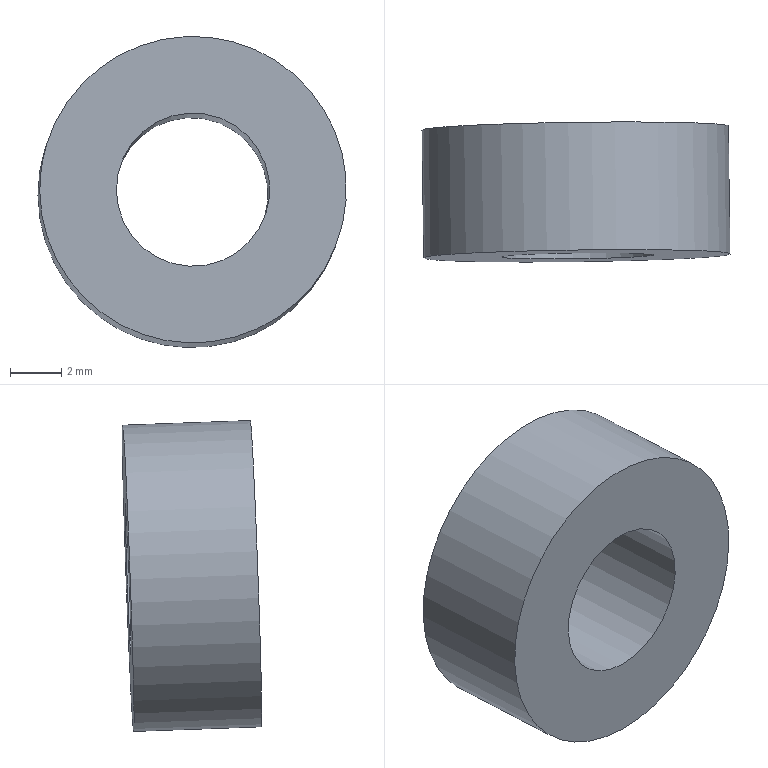Part | STEP file | Dodanie-wyci_gni_cie1_3 | 1 solid | 4 faces | box 12.066 x 5.461 x 12.174 mm | volume 424.115 mm3 | cylinder 2 | plane 2 | commonest cylinder face diameters 6 x1 12 x1
STEP:
#1=CARTESIAN_POINT('',(0.,0.,0.));
#2=DIRECTION('',(0.,0.,1.));
#3=DIRECTION('',(1.,0.,0.));
#4=AXIS2_PLACEMENT_3D('',#1,#2,#3);
#5=CARTESIAN_POINT('',(-105.684,187.779,-123.973));
#6=VERTEX_POINT('',#5);
#7=CARTESIAN_POINT('',(-105.752,192.775,-124.155));
#8=VERTEX_POINT('',#7);
#9=CARTESIAN_POINT('',(-105.684,187.779,-123.973));
#10=DIRECTION('',(-0.01351,0.9992,-0.0363));
#11=VECTOR('',#10,1.);
#12=LINE('',#9,#11);
#13=CARTESIAN_POINT('',(-99.753,192.858,-124.114));
#14=DIRECTION('',(0.01351,-0.9992,0.0363));
#15=DIRECTION('',(-0.9999,-0.01377,-0.006861));
#16=AXIS2_PLACEMENT_3D('',#13,#14,#15);
#17=CYLINDRICAL_SURFACE('',#16,6.);
#18=CARTESIAN_POINT('',(0.,5.));
#19=DIRECTION('',(0.,-1.));
#20=VECTOR('',#19,1.);
#21=LINE('',#18,#20);
#22=(GEOMETRIC_REPRESENTATION_CONTEXT(2)PARAMETRIC_REPRESENTATION_CONTEXT()REPRESENTATION_CONTEXT('',''));
#23=DEFINITIONAL_REPRESENTATION('',(#21),#22);
#24=PCURVE('',#17,#23);
#25=CARTESIAN_POINT('',(6.283,5.));
#26=DIRECTION('',(0.,-1.));
#27=VECTOR('',#26,1.);
#28=LINE('',#25,#27);
#29=(GEOMETRIC_REPRESENTATION_CONTEXT(2)PARAMETRIC_REPRESENTATION_CONTEXT()REPRESENTATION_CONTEXT('',''));
#30=DEFINITIONAL_REPRESENTATION('',(#28),#29);
#31=PCURVE('',#17,#30);
#32=SEAM_CURVE('',#12,(#24,#31),.PCURVE_S1.);
#33=EDGE_CURVE('',#6,#8,#32,.T.);
#34=ORIENTED_EDGE('',*,*,#33,.T.);
#35=CARTESIAN_POINT('',(-99.753,192.858,-124.114));
#36=DIRECTION('',(0.01351,-0.9992,0.0363));
#37=DIRECTION('',(-0.9999,-0.01377,-0.006861));
#38=AXIS2_PLACEMENT_3D('',#35,#36,#37);
#39=CIRCLE('',#38,6.);
#40=CARTESIAN_POINT('',(0.,0.));
#41=DIRECTION('',(1.,0.));
#42=VECTOR('',#41,1.);
#43=LINE('',#40,#42);
#44=(GEOMETRIC_REPRESENTATION_CONTEXT(2)PARAMETRIC_REPRESENTATION_CONTEXT()REPRESENTATION_CONTEXT('',''));
#45=DEFINITIONAL_REPRESENTATION('',(#43),#44);
#46=PCURVE('',#17,#45);
#47=CARTESIAN_POINT('',(-99.753,192.858,-124.114));
#48=DIRECTION('',(-0.01351,0.9992,-0.0363));
#49=DIRECTION('',(0.9999,0.01377,0.006861));
#50=AXIS2_PLACEMENT_3D('',#47,#48,#49);
#51=PLANE('',#50);
#52=CARTESIAN_POINT('',(-6.,0.));
#53=CARTESIAN_POINT('',(-6.,10.392));
#54=CARTESIAN_POINT('',(3.,5.196));
#55=CARTESIAN_POINT('',(12.,0.));
#56=CARTESIAN_POINT('',(3.,-5.196));
#57=CARTESIAN_POINT('',(-6.,-10.392));
#58=CARTESIAN_POINT('',(-6.,0.));
#59=(BOUNDED_CURVE()B_SPLINE_CURVE(2,(#52,#53,#54,#55,#56,#57,#58),.UNSPECIFIED.,.T.,.F.)B_SPLINE_CURVE_WITH_KNOTS((1,2,2,2,2,1),(-2.094,0.,2.094,4.189,6.283,8.378),.UNSPECIFIED.)CURVE()GEOMETRIC_REPRESENTATION_ITEM()RATIONAL_B_SPLINE_CURVE((1.,0.5,1.,0.5,1.,0.5,1.))REPRESENTATION_ITEM(''));
#60=(GEOMETRIC_REPRESENTATION_CONTEXT(2)PARAMETRIC_REPRESENTATION_CONTEXT()REPRESENTATION_CONTEXT('',''));
#61=DEFINITIONAL_REPRESENTATION('',(#59),#60);
#62=PCURVE('',#51,#61);
#63=SURFACE_CURVE('',#39,(#46,#62),.PCURVE_S1.);
#64=EDGE_CURVE('',#8,#8,#63,.T.);
#65=ORIENTED_EDGE('',*,*,#64,.T.);
#66=ORIENTED_EDGE('',*,*,#33,.F.);
#67=CARTESIAN_POINT('',(-99.685,187.862,-123.932));
#68=DIRECTION('',(-0.01351,0.9992,-0.0363));
#69=DIRECTION('',(-0.9999,-0.01377,-0.006861));
#70=AXIS2_PLACEMENT_3D('',#67,#68,#69);
#71=CIRCLE('',#70,6.);
#72=CARTESIAN_POINT('',(6.283,5.));
#73=DIRECTION('',(-1.,0.));
#74=VECTOR('',#73,1.);
#75=LINE('',#72,#74);
#76=(GEOMETRIC_REPRESENTATION_CONTEXT(2)PARAMETRIC_REPRESENTATION_CONTEXT()REPRESENTATION_CONTEXT('',''));
#77=DEFINITIONAL_REPRESENTATION('',(#75),#76);
#78=PCURVE('',#17,#77);
#79=CARTESIAN_POINT('',(-99.685,187.862,-123.932));
#80=DIRECTION('',(-0.01351,0.9992,-0.0363));
#81=DIRECTION('',(0.9999,0.01377,0.006861));
#82=AXIS2_PLACEMENT_3D('',#79,#80,#81);
#83=PLANE('',#82);
#84=CARTESIAN_POINT('',(0.,0.));
#85=DIRECTION('',(-1.,0.));
#86=AXIS2_PLACEMENT_2D('',#84,#85);
#87=CIRCLE('',#86,6.);
#88=(GEOMETRIC_REPRESENTATION_CONTEXT(2)PARAMETRIC_REPRESENTATION_CONTEXT()REPRESENTATION_CONTEXT('',''));
#89=DEFINITIONAL_REPRESENTATION('',(#87),#88);
#90=PCURVE('',#83,#89);
#91=SURFACE_CURVE('',#71,(#78,#90),.PCURVE_S1.);
#92=EDGE_CURVE('',#6,#6,#91,.T.);
#93=ORIENTED_EDGE('',*,*,#92,.T.);
#94=EDGE_LOOP('',(#34,#65,#66,#93));
#95=FACE_BOUND('',#94,.T.);
#96=ADVANCED_FACE('',(#95),#17,.T.);
#97=CARTESIAN_POINT('',(-102.752,192.817,-124.134));
#98=VERTEX_POINT('',#97);
#99=CARTESIAN_POINT('',(-99.753,192.858,-124.114));
#100=DIRECTION('',(0.01351,-0.9992,0.0363));
#101=DIRECTION('',(-0.9999,-0.01377,-0.006861));
#102=AXIS2_PLACEMENT_3D('',#99,#100,#101);
#103=CIRCLE('',#102,3.);
#104=CARTESIAN_POINT('',(-99.753,192.858,-124.114));
#105=DIRECTION('',(0.01351,-0.9992,0.0363));
#106=DIRECTION('',(-0.9999,-0.01377,-0.006861));
#107=AXIS2_PLACEMENT_3D('',#104,#105,#106);
#108=CYLINDRICAL_SURFACE('',#107,3.);
#109=CARTESIAN_POINT('',(0.,0.));
#110=DIRECTION('',(1.,0.));
#111=VECTOR('',#110,1.);
#112=LINE('',#109,#111);
#113=(GEOMETRIC_REPRESENTATION_CONTEXT(2)PARAMETRIC_REPRESENTATION_CONTEXT()REPRESENTATION_CONTEXT('',''));
#114=DEFINITIONAL_REPRESENTATION('',(#112),#113);
#115=PCURVE('',#108,#114);
#116=CARTESIAN_POINT('',(-3.,0.));
#117=CARTESIAN_POINT('',(-3.,5.196));
#118=CARTESIAN_POINT('',(1.5,2.598));
#119=CARTESIAN_POINT('',(6.,0.));
#120=CARTESIAN_POINT('',(1.5,-2.598));
#121=CARTESIAN_POINT('',(-3.,-5.196));
#122=CARTESIAN_POINT('',(-3.,0.));
#123=(BOUNDED_CURVE()B_SPLINE_CURVE(2,(#116,#117,#118,#119,#120,#121,#122),.UNSPECIFIED.,.T.,.F.)B_SPLINE_CURVE_WITH_KNOTS((1,2,2,2,2,1),(-2.094,0.,2.094,4.189,6.283,8.378),.UNSPECIFIED.)CURVE()GEOMETRIC_REPRESENTATION_ITEM()RATIONAL_B_SPLINE_CURVE((1.,0.5,1.,0.5,1.,0.5,1.))REPRESENTATION_ITEM(''));
#124=(GEOMETRIC_REPRESENTATION_CONTEXT(2)PARAMETRIC_REPRESENTATION_CONTEXT()REPRESENTATION_CONTEXT('',''));
#125=DEFINITIONAL_REPRESENTATION('',(#123),#124);
#126=PCURVE('',#51,#125);
#127=SURFACE_CURVE('',#103,(#115,#126),.PCURVE_S1.);
#128=EDGE_CURVE('',#98,#98,#127,.T.);
#129=ORIENTED_EDGE('',*,*,#128,.T.);
#130=CARTESIAN_POINT('',(-102.685,187.821,-123.953));
#131=VERTEX_POINT('',#130);
#132=CARTESIAN_POINT('',(-102.685,187.821,-123.953));
#133=DIRECTION('',(-0.01351,0.9992,-0.0363));
#134=VECTOR('',#133,1.);
#135=LINE('',#132,#134);
#136=CARTESIAN_POINT('',(6.283,5.));
#137=DIRECTION('',(0.,-1.));
#138=VECTOR('',#137,1.);
#139=LINE('',#136,#138);
#140=(GEOMETRIC_REPRESENTATION_CONTEXT(2)PARAMETRIC_REPRESENTATION_CONTEXT()REPRESENTATION_CONTEXT('',''));
#141=DEFINITIONAL_REPRESENTATION('',(#139),#140);
#142=PCURVE('',#108,#141);
#143=CARTESIAN_POINT('',(0.,5.));
#144=DIRECTION('',(0.,-1.));
#145=VECTOR('',#144,1.);
#146=LINE('',#143,#145);
#147=(GEOMETRIC_REPRESENTATION_CONTEXT(2)PARAMETRIC_REPRESENTATION_CONTEXT()REPRESENTATION_CONTEXT('',''));
#148=DEFINITIONAL_REPRESENTATION('',(#146),#147);
#149=PCURVE('',#108,#148);
#150=SEAM_CURVE('',#135,(#142,#149),.PCURVE_S1.);
#151=EDGE_CURVE('',#131,#98,#150,.T.);
#152=ORIENTED_EDGE('',*,*,#151,.F.);
#153=CARTESIAN_POINT('',(-99.685,187.862,-123.932));
#154=DIRECTION('',(0.01351,-0.9992,0.0363));
#155=DIRECTION('',(-0.9999,-0.01377,-0.006861));
#156=AXIS2_PLACEMENT_3D('',#153,#154,#155);
#157=CIRCLE('',#156,3.);
#158=CARTESIAN_POINT('',(0.,5.));
#159=DIRECTION('',(1.,0.));
#160=VECTOR('',#159,1.);
#161=LINE('',#158,#160);
#162=(GEOMETRIC_REPRESENTATION_CONTEXT(2)PARAMETRIC_REPRESENTATION_CONTEXT()REPRESENTATION_CONTEXT('',''));
#163=DEFINITIONAL_REPRESENTATION('',(#161),#162);
#164=PCURVE('',#108,#163);
#165=CARTESIAN_POINT('',(-3.,0.));
#166=CARTESIAN_POINT('',(-3.,5.196));
#167=CARTESIAN_POINT('',(1.5,2.598));
#168=CARTESIAN_POINT('',(6.,0.));
#169=CARTESIAN_POINT('',(1.5,-2.598));
#170=CARTESIAN_POINT('',(-3.,-5.196));
#171=CARTESIAN_POINT('',(-3.,0.));
#172=(BOUNDED_CURVE()B_SPLINE_CURVE(2,(#165,#166,#167,#168,#169,#170,#171),.UNSPECIFIED.,.T.,.F.)B_SPLINE_CURVE_WITH_KNOTS((1,2,2,2,2,1),(-2.094,0.,2.094,4.189,6.283,8.378),.UNSPECIFIED.)CURVE()GEOMETRIC_REPRESENTATION_ITEM()RATIONAL_B_SPLINE_CURVE((1.,0.5,1.,0.5,1.,0.5,1.))REPRESENTATION_ITEM(''));
#173=(GEOMETRIC_REPRESENTATION_CONTEXT(2)PARAMETRIC_REPRESENTATION_CONTEXT()REPRESENTATION_CONTEXT('',''));
#174=DEFINITIONAL_REPRESENTATION('',(#172),#173);
#175=PCURVE('',#83,#174);
#176=SURFACE_CURVE('',#157,(#164,#175),.PCURVE_S1.);
#177=EDGE_CURVE('',#131,#131,#176,.T.);
#178=ORIENTED_EDGE('',*,*,#177,.F.);
#179=ORIENTED_EDGE('',*,*,#151,.T.);
#180=EDGE_LOOP('',(#129,#152,#178,#179));
#181=FACE_BOUND('',#180,.F.);
#182=ADVANCED_FACE('',(#181),#108,.F.);
#183=ORIENTED_EDGE('',*,*,#177,.F.);
#184=EDGE_LOOP('',(#183));
#185=FACE_BOUND('',#184,.T.);
#186=ORIENTED_EDGE('',*,*,#92,.F.);
#187=EDGE_LOOP('',(#186));
#188=FACE_BOUND('',#187,.T.);
#189=ADVANCED_FACE('',(#185,#188),#83,.F.);
#190=ORIENTED_EDGE('',*,*,#128,.T.);
#191=EDGE_LOOP('',(#190));
#192=FACE_BOUND('',#191,.T.);
#193=ORIENTED_EDGE('',*,*,#64,.F.);
#194=EDGE_LOOP('',(#193));
#195=FACE_BOUND('',#194,.T.);
#196=ADVANCED_FACE('',(#192,#195),#51,.T.);
#197=CLOSED_SHELL('',(#96,#182,#189,#196));
#198=MANIFOLD_SOLID_BREP('',#197);
#199=(LENGTH_UNIT()NAMED_UNIT(*)SI_UNIT(.MILLI.,.METRE.));
#200=UNCERTAINTY_MEASURE_WITH_UNIT(LENGTH_MEASURE(0.0000001),#199,'','');
#201=(NAMED_UNIT(*)PLANE_ANGLE_UNIT()SI_UNIT($,.RADIAN.));
#202=(NAMED_UNIT(*)SI_UNIT($,.STERADIAN.)SOLID_ANGLE_UNIT());
#203=(GEOMETRIC_REPRESENTATION_CONTEXT(3)GLOBAL_UNCERTAINTY_ASSIGNED_CONTEXT((#200))GLOBAL_UNIT_ASSIGNED_CONTEXT((#199,#201,#202))REPRESENTATION_CONTEXT('',''));
#204=ADVANCED_BREP_SHAPE_REPRESENTATION('',(#4,#198),#203);